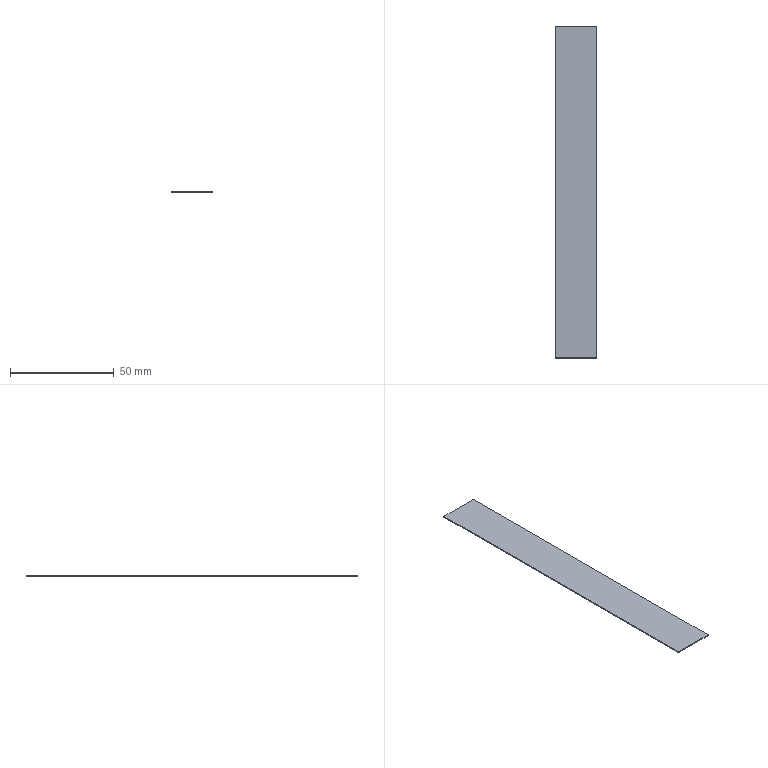Part | NX | 1 solid | 6 faces | box 20 x 160 x 0.5 mm | volume 1600 mm3 | plane 6
STEP:
#1=CARTESIAN_POINT('',(12.5,-95.,1.));
#2=VERTEX_POINT('',#1);
#3=CARTESIAN_POINT('',(12.5,-255.,1.));
#4=VERTEX_POINT('',#3);
#5=CARTESIAN_POINT('',(12.5,-95.,1.));
#6=DIRECTION('',(0.,-1.,0.));
#7=VECTOR('',#6,1000.);
#8=LINE('',#5,#7);
#9=EDGE_CURVE('',#2,#4,#8,.T.);
#10=ORIENTED_EDGE('',*,*,#9,.T.);
#11=CARTESIAN_POINT('',(12.5,-255.,1.5));
#12=VERTEX_POINT('',#11);
#13=CARTESIAN_POINT('',(12.5,-255.,1.5));
#14=DIRECTION('',(0.,0.,-1.));
#15=VECTOR('',#14,1000.);
#16=LINE('',#13,#15);
#17=EDGE_CURVE('',#12,#4,#16,.T.);
#18=ORIENTED_EDGE('',*,*,#17,.F.);
#19=CARTESIAN_POINT('',(12.5,-95.,1.5));
#20=VERTEX_POINT('',#19);
#21=CARTESIAN_POINT('',(12.5,-95.,1.5));
#22=DIRECTION('',(0.,-1.,0.));
#23=VECTOR('',#22,1000.);
#24=LINE('',#21,#23);
#25=EDGE_CURVE('',#20,#12,#24,.T.);
#26=ORIENTED_EDGE('',*,*,#25,.F.);
#27=CARTESIAN_POINT('',(12.5,-95.,1.5));
#28=DIRECTION('',(0.,0.,-1.));
#29=VECTOR('',#28,1000.);
#30=LINE('',#27,#29);
#31=EDGE_CURVE('',#20,#2,#30,.T.);
#32=ORIENTED_EDGE('',*,*,#31,.T.);
#33=EDGE_LOOP('',(#10,#18,#26,#32));
#34=FACE_BOUND('',#33,.T.);
#35=CARTESIAN_POINT('',(12.5,-95.,1.5));
#36=DIRECTION('',(1.,0.,0.));
#37=DIRECTION('',(0.,1.,0.));
#38=AXIS2_PLACEMENT_3D('',#35,#36,#37);
#39=PLANE('',#38);
#40=ADVANCED_FACE('',(#34),#39,.F.);
#41=CARTESIAN_POINT('',(32.5,-255.,1.));
#42=VERTEX_POINT('',#41);
#43=CARTESIAN_POINT('',(12.5,-255.,1.));
#44=DIRECTION('',(1.,0.,0.));
#45=VECTOR('',#44,1000.);
#46=LINE('',#43,#45);
#47=EDGE_CURVE('',#4,#42,#46,.T.);
#48=ORIENTED_EDGE('',*,*,#47,.T.);
#49=CARTESIAN_POINT('',(32.5,-255.,1.5));
#50=VERTEX_POINT('',#49);
#51=CARTESIAN_POINT('',(32.5,-255.,1.5));
#52=DIRECTION('',(0.,0.,-1.));
#53=VECTOR('',#52,1000.);
#54=LINE('',#51,#53);
#55=EDGE_CURVE('',#50,#42,#54,.T.);
#56=ORIENTED_EDGE('',*,*,#55,.F.);
#57=CARTESIAN_POINT('',(12.5,-255.,1.5));
#58=DIRECTION('',(1.,0.,0.));
#59=VECTOR('',#58,1000.);
#60=LINE('',#57,#59);
#61=EDGE_CURVE('',#12,#50,#60,.T.);
#62=ORIENTED_EDGE('',*,*,#61,.F.);
#63=ORIENTED_EDGE('',*,*,#17,.T.);
#64=EDGE_LOOP('',(#48,#56,#62,#63));
#65=FACE_BOUND('',#64,.T.);
#66=CARTESIAN_POINT('',(12.5,-255.,1.5));
#67=DIRECTION('',(0.,1.,0.));
#68=DIRECTION('',(0.,0.,1.));
#69=AXIS2_PLACEMENT_3D('',#66,#67,#68);
#70=PLANE('',#69);
#71=ADVANCED_FACE('',(#65),#70,.F.);
#72=CARTESIAN_POINT('',(32.5,-95.,1.));
#73=VERTEX_POINT('',#72);
#74=CARTESIAN_POINT('',(32.5,-95.,1.));
#75=DIRECTION('',(0.,1.,0.));
#76=VECTOR('',#75,1000.);
#77=LINE('',#74,#76);
#78=EDGE_CURVE('',#42,#73,#77,.T.);
#79=ORIENTED_EDGE('',*,*,#78,.T.);
#80=CARTESIAN_POINT('',(32.5,-95.,1.5));
#81=VERTEX_POINT('',#80);
#82=CARTESIAN_POINT('',(32.5,-95.,1.5));
#83=DIRECTION('',(0.,0.,-1.));
#84=VECTOR('',#83,1000.);
#85=LINE('',#82,#84);
#86=EDGE_CURVE('',#81,#73,#85,.T.);
#87=ORIENTED_EDGE('',*,*,#86,.F.);
#88=CARTESIAN_POINT('',(32.5,-95.,1.5));
#89=DIRECTION('',(0.,1.,0.));
#90=VECTOR('',#89,1000.);
#91=LINE('',#88,#90);
#92=EDGE_CURVE('',#50,#81,#91,.T.);
#93=ORIENTED_EDGE('',*,*,#92,.F.);
#94=ORIENTED_EDGE('',*,*,#55,.T.);
#95=EDGE_LOOP('',(#79,#87,#93,#94));
#96=FACE_BOUND('',#95,.T.);
#97=CARTESIAN_POINT('',(32.5,-95.,1.5));
#98=DIRECTION('',(-1.,0.,0.));
#99=DIRECTION('',(0.,-1.,0.));
#100=AXIS2_PLACEMENT_3D('',#97,#98,#99);
#101=PLANE('',#100);
#102=ADVANCED_FACE('',(#96),#101,.F.);
#103=CARTESIAN_POINT('',(12.5,-95.,1.));
#104=DIRECTION('',(-1.,0.,0.));
#105=VECTOR('',#104,1000.);
#106=LINE('',#103,#105);
#107=EDGE_CURVE('',#73,#2,#106,.T.);
#108=ORIENTED_EDGE('',*,*,#107,.T.);
#109=ORIENTED_EDGE('',*,*,#31,.F.);
#110=CARTESIAN_POINT('',(12.5,-95.,1.5));
#111=DIRECTION('',(-1.,0.,0.));
#112=VECTOR('',#111,1000.);
#113=LINE('',#110,#112);
#114=EDGE_CURVE('',#81,#20,#113,.T.);
#115=ORIENTED_EDGE('',*,*,#114,.F.);
#116=ORIENTED_EDGE('',*,*,#86,.T.);
#117=EDGE_LOOP('',(#108,#109,#115,#116));
#118=FACE_BOUND('',#117,.T.);
#119=CARTESIAN_POINT('',(12.5,-95.,1.5));
#120=DIRECTION('',(0.,-1.,0.));
#121=DIRECTION('',(0.,0.,-1.));
#122=AXIS2_PLACEMENT_3D('',#119,#120,#121);
#123=PLANE('',#122);
#124=ADVANCED_FACE('',(#118),#123,.F.);
#125=ORIENTED_EDGE('',*,*,#25,.T.);
#126=ORIENTED_EDGE('',*,*,#61,.T.);
#127=ORIENTED_EDGE('',*,*,#92,.T.);
#128=ORIENTED_EDGE('',*,*,#114,.T.);
#129=EDGE_LOOP('',(#125,#126,#127,#128));
#130=FACE_BOUND('',#129,.T.);
#131=CARTESIAN_POINT('',(0.,0.,1.5));
#132=DIRECTION('',(0.,0.,1.));
#133=DIRECTION('',(1.,0.,0.));
#134=AXIS2_PLACEMENT_3D('',#131,#132,#133);
#135=PLANE('',#134);
#136=ADVANCED_FACE('',(#130),#135,.T.);
#137=ORIENTED_EDGE('',*,*,#9,.F.);
#138=ORIENTED_EDGE('',*,*,#107,.F.);
#139=ORIENTED_EDGE('',*,*,#78,.F.);
#140=ORIENTED_EDGE('',*,*,#47,.F.);
#141=EDGE_LOOP('',(#137,#138,#139,#140));
#142=FACE_BOUND('',#141,.T.);
#143=CARTESIAN_POINT('',(0.,0.,1.));
#144=DIRECTION('',(0.,0.,1.));
#145=DIRECTION('',(1.,0.,0.));
#146=AXIS2_PLACEMENT_3D('',#143,#144,#145);
#147=PLANE('',#146);
#148=ADVANCED_FACE('',(#142),#147,.F.);
#149=CLOSED_SHELL('',(#40,#71,#102,#124,#136,#148));
#150=MANIFOLD_SOLID_BREP('',#149);
#151=(LENGTH_UNIT()NAMED_UNIT(*)SI_UNIT(.MILLI.,.METRE.));
#152=UNCERTAINTY_MEASURE_WITH_UNIT(LENGTH_MEASURE(0.00001),#151,'','');
#153=(NAMED_UNIT(*)PLANE_ANGLE_UNIT()SI_UNIT($,.RADIAN.));
#154=(NAMED_UNIT(*)SI_UNIT($,.STERADIAN.)SOLID_ANGLE_UNIT());
#155=(GEOMETRIC_REPRESENTATION_CONTEXT(3)GLOBAL_UNCERTAINTY_ASSIGNED_CONTEXT((#152))GLOBAL_UNIT_ASSIGNED_CONTEXT((#151,#153,#154))REPRESENTATION_CONTEXT('',''));
#156=ADVANCED_BREP_SHAPE_REPRESENTATION('',(#150),#155);